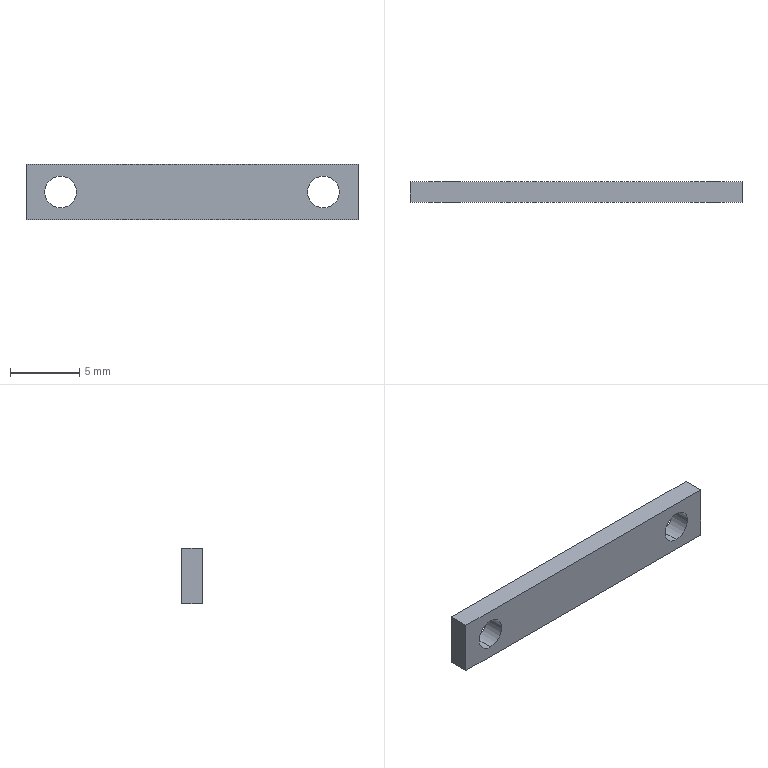Part | SolidWorks | features Extrusion 1, HoleWzd 1 | 1 solid | 10 faces | box 24 x 1.5 x 4 mm | volume 131.536 mm3 | plane 6 | cylinder 4 | commonest cylinder face diameters 2.3 x4
STEP:
#1=CARTESIAN_POINT('',(-9.5,-0.75,-1.15));
#2=VERTEX_POINT('',#1);
#3=CARTESIAN_POINT('',(-9.5,-0.75,1.15));
#4=VERTEX_POINT('',#3);
#5=CARTESIAN_POINT('',(-9.5,-0.75,0.));
#6=DIRECTION('',(0.,1.,0.));
#7=DIRECTION('',(0.,0.,1.));
#8=AXIS2_PLACEMENT_3D('',#5,#6,#7);
#9=CIRCLE('',#8,1.15);
#10=EDGE_CURVE('',#2,#4,#9,.T.);
#11=ORIENTED_EDGE('',*,*,#10,.F.);
#12=CARTESIAN_POINT('',(-9.5,0.75,-1.15));
#13=VERTEX_POINT('',#12);
#14=CARTESIAN_POINT('',(-9.5,0.75,-1.15));
#15=DIRECTION('',(0.,1.,0.));
#16=VECTOR('',#15,1000.);
#17=LINE('',#14,#16);
#18=EDGE_CURVE('',#2,#13,#17,.T.);
#19=ORIENTED_EDGE('',*,*,#18,.T.);
#20=CARTESIAN_POINT('',(-9.5,0.75,1.15));
#21=VERTEX_POINT('',#20);
#22=CARTESIAN_POINT('',(-9.5,0.75,0.));
#23=DIRECTION('',(0.,1.,0.));
#24=DIRECTION('',(0.,0.,1.));
#25=AXIS2_PLACEMENT_3D('',#22,#23,#24);
#26=CIRCLE('',#25,1.15);
#27=EDGE_CURVE('',#13,#21,#26,.T.);
#28=ORIENTED_EDGE('',*,*,#27,.T.);
#29=CARTESIAN_POINT('',(-9.5,0.75,1.15));
#30=DIRECTION('',(0.,1.,0.));
#31=VECTOR('',#30,1000.);
#32=LINE('',#29,#31);
#33=EDGE_CURVE('',#4,#21,#32,.T.);
#34=ORIENTED_EDGE('',*,*,#33,.F.);
#35=EDGE_LOOP('',(#11,#19,#28,#34));
#36=FACE_OUTER_BOUND('',#35,.T.);
#37=CARTESIAN_POINT('',(-9.5,0.75,0.));
#38=DIRECTION('',(0.,1.,0.));
#39=DIRECTION('',(0.,0.,1.));
#40=AXIS2_PLACEMENT_3D('',#37,#38,#39);
#41=CYLINDRICAL_SURFACE('',#40,1.15);
#42=ADVANCED_FACE('',(#36),#41,.F.);
#43=CARTESIAN_POINT('',(9.5,-0.75,-1.15));
#44=VERTEX_POINT('',#43);
#45=CARTESIAN_POINT('',(9.5,-0.75,1.15));
#46=VERTEX_POINT('',#45);
#47=CARTESIAN_POINT('',(9.5,-0.75,0.));
#48=DIRECTION('',(0.,1.,0.));
#49=DIRECTION('',(0.,0.,1.));
#50=AXIS2_PLACEMENT_3D('',#47,#48,#49);
#51=CIRCLE('',#50,1.15);
#52=EDGE_CURVE('',#44,#46,#51,.T.);
#53=ORIENTED_EDGE('',*,*,#52,.F.);
#54=CARTESIAN_POINT('',(9.5,0.75,-1.15));
#55=VERTEX_POINT('',#54);
#56=CARTESIAN_POINT('',(9.5,0.75,-1.15));
#57=DIRECTION('',(0.,1.,0.));
#58=VECTOR('',#57,1000.);
#59=LINE('',#56,#58);
#60=EDGE_CURVE('',#44,#55,#59,.T.);
#61=ORIENTED_EDGE('',*,*,#60,.T.);
#62=CARTESIAN_POINT('',(9.5,0.75,1.15));
#63=VERTEX_POINT('',#62);
#64=CARTESIAN_POINT('',(9.5,0.75,0.));
#65=DIRECTION('',(0.,1.,0.));
#66=DIRECTION('',(0.,0.,1.));
#67=AXIS2_PLACEMENT_3D('',#64,#65,#66);
#68=CIRCLE('',#67,1.15);
#69=EDGE_CURVE('',#55,#63,#68,.T.);
#70=ORIENTED_EDGE('',*,*,#69,.T.);
#71=CARTESIAN_POINT('',(9.5,0.75,1.15));
#72=DIRECTION('',(0.,1.,0.));
#73=VECTOR('',#72,1000.);
#74=LINE('',#71,#73);
#75=EDGE_CURVE('',#46,#63,#74,.T.);
#76=ORIENTED_EDGE('',*,*,#75,.F.);
#77=EDGE_LOOP('',(#53,#61,#70,#76));
#78=FACE_OUTER_BOUND('',#77,.T.);
#79=CARTESIAN_POINT('',(9.5,0.75,0.));
#80=DIRECTION('',(0.,1.,0.));
#81=DIRECTION('',(0.,0.,1.));
#82=AXIS2_PLACEMENT_3D('',#79,#80,#81);
#83=CYLINDRICAL_SURFACE('',#82,1.15);
#84=ADVANCED_FACE('',(#78),#83,.F.);
#85=CARTESIAN_POINT('',(12.,-0.75,2.));
#86=VERTEX_POINT('',#85);
#87=CARTESIAN_POINT('',(12.,-0.75,-2.));
#88=VERTEX_POINT('',#87);
#89=CARTESIAN_POINT('',(12.,-0.75,-2.));
#90=DIRECTION('',(0.,0.,-1.));
#91=VECTOR('',#90,1000.);
#92=LINE('',#89,#91);
#93=EDGE_CURVE('',#86,#88,#92,.T.);
#94=ORIENTED_EDGE('',*,*,#93,.T.);
#95=CARTESIAN_POINT('',(12.,0.75,-2.));
#96=VERTEX_POINT('',#95);
#97=CARTESIAN_POINT('',(12.,0.75,-2.));
#98=DIRECTION('',(0.,-1.,0.));
#99=VECTOR('',#98,1000.);
#100=LINE('',#97,#99);
#101=EDGE_CURVE('',#96,#88,#100,.T.);
#102=ORIENTED_EDGE('',*,*,#101,.F.);
#103=CARTESIAN_POINT('',(12.,0.75,2.));
#104=VERTEX_POINT('',#103);
#105=CARTESIAN_POINT('',(12.,0.75,-2.));
#106=DIRECTION('',(0.,0.,-1.));
#107=VECTOR('',#106,1000.);
#108=LINE('',#105,#107);
#109=EDGE_CURVE('',#104,#96,#108,.T.);
#110=ORIENTED_EDGE('',*,*,#109,.F.);
#111=CARTESIAN_POINT('',(12.,0.75,2.));
#112=DIRECTION('',(0.,-1.,0.));
#113=VECTOR('',#112,1000.);
#114=LINE('',#111,#113);
#115=EDGE_CURVE('',#104,#86,#114,.T.);
#116=ORIENTED_EDGE('',*,*,#115,.T.);
#117=EDGE_LOOP('',(#94,#102,#110,#116));
#118=FACE_OUTER_BOUND('',#117,.T.);
#119=CARTESIAN_POINT('',(12.,0.75,-2.));
#120=DIRECTION('',(-1.,0.,0.));
#121=DIRECTION('',(0.,0.,1.));
#122=AXIS2_PLACEMENT_3D('',#119,#120,#121);
#123=PLANE('',#122);
#124=ADVANCED_FACE('',(#118),#123,.F.);
#125=CARTESIAN_POINT('',(-12.,-0.75,-2.));
#126=VERTEX_POINT('',#125);
#127=CARTESIAN_POINT('',(-12.,-0.75,-2.));
#128=DIRECTION('',(-1.,0.,0.));
#129=VECTOR('',#128,1000.);
#130=LINE('',#127,#129);
#131=EDGE_CURVE('',#88,#126,#130,.T.);
#132=ORIENTED_EDGE('',*,*,#131,.T.);
#133=CARTESIAN_POINT('',(-12.,0.75,-2.));
#134=VERTEX_POINT('',#133);
#135=CARTESIAN_POINT('',(-12.,0.75,-2.));
#136=DIRECTION('',(0.,-1.,0.));
#137=VECTOR('',#136,1000.);
#138=LINE('',#135,#137);
#139=EDGE_CURVE('',#134,#126,#138,.T.);
#140=ORIENTED_EDGE('',*,*,#139,.F.);
#141=CARTESIAN_POINT('',(-12.,0.75,-2.));
#142=DIRECTION('',(-1.,0.,0.));
#143=VECTOR('',#142,1000.);
#144=LINE('',#141,#143);
#145=EDGE_CURVE('',#96,#134,#144,.T.);
#146=ORIENTED_EDGE('',*,*,#145,.F.);
#147=ORIENTED_EDGE('',*,*,#101,.T.);
#148=EDGE_LOOP('',(#132,#140,#146,#147));
#149=FACE_OUTER_BOUND('',#148,.T.);
#150=CARTESIAN_POINT('',(-12.,0.75,-2.));
#151=DIRECTION('',(0.,0.,1.));
#152=DIRECTION('',(1.,0.,0.));
#153=AXIS2_PLACEMENT_3D('',#150,#151,#152);
#154=PLANE('',#153);
#155=ADVANCED_FACE('',(#149),#154,.F.);
#156=CARTESIAN_POINT('',(-12.,-0.75,2.));
#157=VERTEX_POINT('',#156);
#158=CARTESIAN_POINT('',(-12.,-0.75,-2.));
#159=DIRECTION('',(0.,0.,1.));
#160=VECTOR('',#159,1000.);
#161=LINE('',#158,#160);
#162=EDGE_CURVE('',#126,#157,#161,.T.);
#163=ORIENTED_EDGE('',*,*,#162,.T.);
#164=CARTESIAN_POINT('',(-12.,0.75,2.));
#165=VERTEX_POINT('',#164);
#166=CARTESIAN_POINT('',(-12.,0.75,2.));
#167=DIRECTION('',(0.,-1.,0.));
#168=VECTOR('',#167,1000.);
#169=LINE('',#166,#168);
#170=EDGE_CURVE('',#165,#157,#169,.T.);
#171=ORIENTED_EDGE('',*,*,#170,.F.);
#172=CARTESIAN_POINT('',(-12.,0.75,-2.));
#173=DIRECTION('',(0.,0.,1.));
#174=VECTOR('',#173,1000.);
#175=LINE('',#172,#174);
#176=EDGE_CURVE('',#134,#165,#175,.T.);
#177=ORIENTED_EDGE('',*,*,#176,.F.);
#178=ORIENTED_EDGE('',*,*,#139,.T.);
#179=EDGE_LOOP('',(#163,#171,#177,#178));
#180=FACE_OUTER_BOUND('',#179,.T.);
#181=CARTESIAN_POINT('',(-12.,0.75,-2.));
#182=DIRECTION('',(1.,0.,0.));
#183=DIRECTION('',(0.,0.,-1.));
#184=AXIS2_PLACEMENT_3D('',#181,#182,#183);
#185=PLANE('',#184);
#186=ADVANCED_FACE('',(#180),#185,.F.);
#187=CARTESIAN_POINT('',(-12.,-0.75,2.));
#188=DIRECTION('',(1.,0.,0.));
#189=VECTOR('',#188,1000.);
#190=LINE('',#187,#189);
#191=EDGE_CURVE('',#157,#86,#190,.T.);
#192=ORIENTED_EDGE('',*,*,#191,.T.);
#193=ORIENTED_EDGE('',*,*,#115,.F.);
#194=CARTESIAN_POINT('',(-12.,0.75,2.));
#195=DIRECTION('',(1.,0.,0.));
#196=VECTOR('',#195,1000.);
#197=LINE('',#194,#196);
#198=EDGE_CURVE('',#165,#104,#197,.T.);
#199=ORIENTED_EDGE('',*,*,#198,.F.);
#200=ORIENTED_EDGE('',*,*,#170,.T.);
#201=EDGE_LOOP('',(#192,#193,#199,#200));
#202=FACE_OUTER_BOUND('',#201,.T.);
#203=CARTESIAN_POINT('',(-12.,0.75,2.));
#204=DIRECTION('',(0.,0.,-1.));
#205=DIRECTION('',(-1.,0.,0.));
#206=AXIS2_PLACEMENT_3D('',#203,#204,#205);
#207=PLANE('',#206);
#208=ADVANCED_FACE('',(#202),#207,.F.);
#209=CARTESIAN_POINT('',(-9.5,0.75,0.));
#210=DIRECTION('',(0.,1.,0.));
#211=DIRECTION('',(0.,0.,1.));
#212=AXIS2_PLACEMENT_3D('',#209,#210,#211);
#213=CIRCLE('',#212,1.15);
#214=EDGE_CURVE('',#21,#13,#213,.T.);
#215=ORIENTED_EDGE('',*,*,#214,.F.);
#216=ORIENTED_EDGE('',*,*,#27,.F.);
#217=EDGE_LOOP('',(#215,#216));
#218=FACE_BOUND('',#217,.T.);
#219=CARTESIAN_POINT('',(9.5,0.75,0.));
#220=DIRECTION('',(0.,1.,0.));
#221=DIRECTION('',(0.,0.,1.));
#222=AXIS2_PLACEMENT_3D('',#219,#220,#221);
#223=CIRCLE('',#222,1.15);
#224=EDGE_CURVE('',#63,#55,#223,.T.);
#225=ORIENTED_EDGE('',*,*,#224,.F.);
#226=ORIENTED_EDGE('',*,*,#69,.F.);
#227=EDGE_LOOP('',(#225,#226));
#228=FACE_BOUND('',#227,.T.);
#229=ORIENTED_EDGE('',*,*,#109,.T.);
#230=ORIENTED_EDGE('',*,*,#145,.T.);
#231=ORIENTED_EDGE('',*,*,#176,.T.);
#232=ORIENTED_EDGE('',*,*,#198,.T.);
#233=EDGE_LOOP('',(#229,#230,#231,#232));
#234=FACE_OUTER_BOUND('',#233,.T.);
#235=CARTESIAN_POINT('',(0.,0.75,0.));
#236=DIRECTION('',(0.,1.,0.));
#237=DIRECTION('',(0.,0.,1.));
#238=AXIS2_PLACEMENT_3D('',#235,#236,#237);
#239=PLANE('',#238);
#240=ADVANCED_FACE('',(#218,#228,#234),#239,.T.);
#241=CARTESIAN_POINT('',(-9.5,-0.75,0.));
#242=DIRECTION('',(0.,1.,0.));
#243=DIRECTION('',(0.,0.,1.));
#244=AXIS2_PLACEMENT_3D('',#241,#242,#243);
#245=CIRCLE('',#244,1.15);
#246=EDGE_CURVE('',#4,#2,#245,.T.);
#247=ORIENTED_EDGE('',*,*,#246,.T.);
#248=ORIENTED_EDGE('',*,*,#10,.T.);
#249=EDGE_LOOP('',(#247,#248));
#250=FACE_BOUND('',#249,.T.);
#251=CARTESIAN_POINT('',(9.5,-0.75,0.));
#252=DIRECTION('',(0.,1.,0.));
#253=DIRECTION('',(0.,0.,1.));
#254=AXIS2_PLACEMENT_3D('',#251,#252,#253);
#255=CIRCLE('',#254,1.15);
#256=EDGE_CURVE('',#46,#44,#255,.T.);
#257=ORIENTED_EDGE('',*,*,#256,.T.);
#258=ORIENTED_EDGE('',*,*,#52,.T.);
#259=EDGE_LOOP('',(#257,#258));
#260=FACE_BOUND('',#259,.T.);
#261=ORIENTED_EDGE('',*,*,#93,.F.);
#262=ORIENTED_EDGE('',*,*,#191,.F.);
#263=ORIENTED_EDGE('',*,*,#162,.F.);
#264=ORIENTED_EDGE('',*,*,#131,.F.);
#265=EDGE_LOOP('',(#261,#262,#263,#264));
#266=FACE_OUTER_BOUND('',#265,.T.);
#267=CARTESIAN_POINT('',(0.,-0.75,0.));
#268=DIRECTION('',(0.,1.,0.));
#269=DIRECTION('',(0.,0.,1.));
#270=AXIS2_PLACEMENT_3D('',#267,#268,#269);
#271=PLANE('',#270);
#272=ADVANCED_FACE('',(#250,#260,#266),#271,.F.);
#273=ORIENTED_EDGE('',*,*,#60,.F.);
#274=ORIENTED_EDGE('',*,*,#256,.F.);
#275=ORIENTED_EDGE('',*,*,#75,.T.);
#276=ORIENTED_EDGE('',*,*,#224,.T.);
#277=EDGE_LOOP('',(#273,#274,#275,#276));
#278=FACE_OUTER_BOUND('',#277,.T.);
#279=CARTESIAN_POINT('',(9.5,0.75,0.));
#280=DIRECTION('',(0.,1.,0.));
#281=DIRECTION('',(0.,0.,1.));
#282=AXIS2_PLACEMENT_3D('',#279,#280,#281);
#283=CYLINDRICAL_SURFACE('',#282,1.15);
#284=ADVANCED_FACE('',(#278),#283,.F.);
#285=ORIENTED_EDGE('',*,*,#18,.F.);
#286=ORIENTED_EDGE('',*,*,#246,.F.);
#287=ORIENTED_EDGE('',*,*,#33,.T.);
#288=ORIENTED_EDGE('',*,*,#214,.T.);
#289=EDGE_LOOP('',(#285,#286,#287,#288));
#290=FACE_OUTER_BOUND('',#289,.T.);
#291=CARTESIAN_POINT('',(-9.5,0.75,0.));
#292=DIRECTION('',(0.,1.,0.));
#293=DIRECTION('',(0.,0.,1.));
#294=AXIS2_PLACEMENT_3D('',#291,#292,#293);
#295=CYLINDRICAL_SURFACE('',#294,1.15);
#296=ADVANCED_FACE('',(#290),#295,.F.);
#297=CLOSED_SHELL('',(#42,#84,#124,#155,#186,#208,#240,#272,#284,#296));
#298=MANIFOLD_SOLID_BREP('',#297);
#299=CARTESIAN_POINT('',(0.,0.,0.));
#300=DIRECTION('',(0.,0.,1.));
#301=DIRECTION('',(1.,0.,0.));
#302=AXIS2_PLACEMENT_3D('',#299,#300,#301);
#303=(LENGTH_UNIT()NAMED_UNIT(*)SI_UNIT(.MILLI.,.METRE.));
#304=UNCERTAINTY_MEASURE_WITH_UNIT(LENGTH_MEASURE(0.00001),#303,'','');
#305=(NAMED_UNIT(*)PLANE_ANGLE_UNIT()SI_UNIT($,.RADIAN.));
#306=(NAMED_UNIT(*)SI_UNIT($,.STERADIAN.)SOLID_ANGLE_UNIT());
#307=(GEOMETRIC_REPRESENTATION_CONTEXT(3)GLOBAL_UNCERTAINTY_ASSIGNED_CONTEXT((#304))GLOBAL_UNIT_ASSIGNED_CONTEXT((#303,#305,#306))REPRESENTATION_CONTEXT('',''));
#308=ADVANCED_BREP_SHAPE_REPRESENTATION('',(#298,#302),#307);